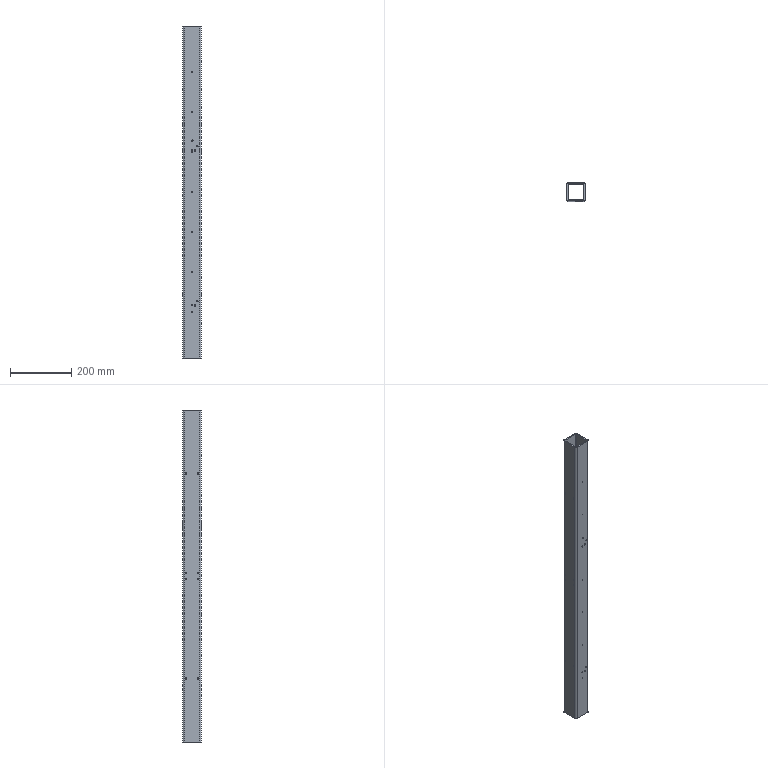Part | STEP file | 1 solid | 104 faces | box 60 x 60 x 1080 mm | volume 942814 mm3 | cylinder 94 | plane 10 | commonest cylinder face diameters 5 x44 3.3 x26 4.2 x16 2 x4 10 x4